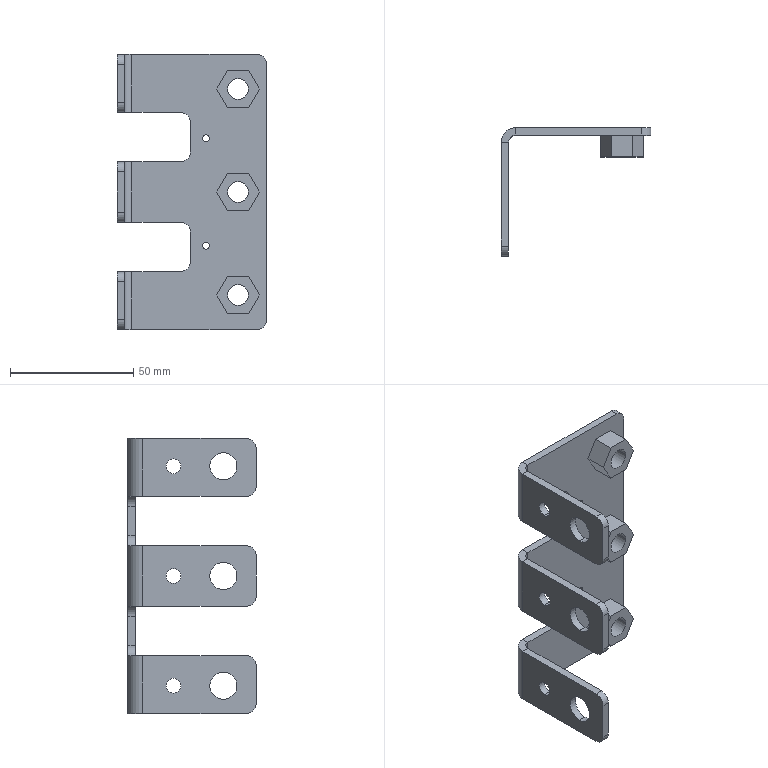Part | STEP file | 64633074 | 1 solid | 93 faces | box 60.788 x 52 x 111.5 mm | volume 28803 mm3 | plane 53 | cylinder 40 | commonest cylinder face diameters 8 x12 6 x9 8.5 x6 11 x6 2.8 x4 12 x3